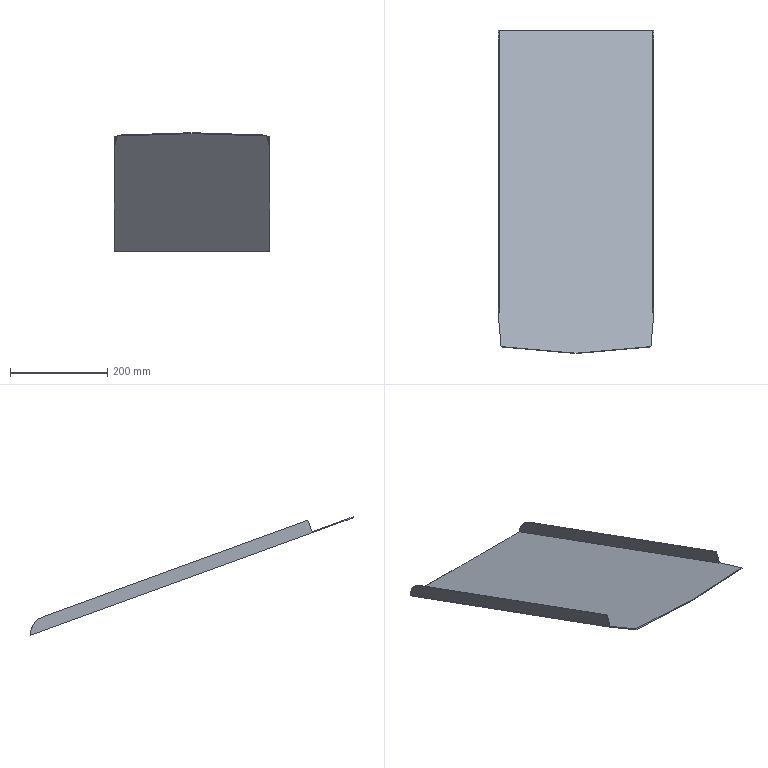Part | NX | features solid 2 | 1 solid | 16 faces | box 320 x 663.823 x 243.491 mm | volume 506723 mm3 | plane 13 | spline 2 | cylinder 1 | commonest cylinder face diameters 80 x1
STEP:
#1=CARTESIAN_POINT('',(160.,49.927,-215.652));
#2=VERTEX_POINT('',#1);
#3=CARTESIAN_POINT('',(158.,49.927,-215.652));
#4=VERTEX_POINT('',#3);
#5=CARTESIAN_POINT('',(160.,49.927,-215.652));
#6=DIRECTION('',(-1.,0.,0.));
#7=VECTOR('',#6,1000.);
#8=LINE('',#5,#7);
#9=EDGE_CURVE('',#2,#4,#8,.T.);
#10=ORIENTED_EDGE('',*,*,#9,.T.);
#11=CARTESIAN_POINT('',(158.,41.376,-239.145));
#12=VERTEX_POINT('',#11);
#13=CARTESIAN_POINT('',(158.,49.927,-215.652));
#14=DIRECTION('',(0.,-0.342,-0.9397));
#15=VECTOR('',#14,1000.);
#16=LINE('',#13,#15);
#17=EDGE_CURVE('',#4,#12,#16,.T.);
#18=ORIENTED_EDGE('',*,*,#17,.T.);
#19=CARTESIAN_POINT('',(160.,41.376,-239.145));
#20=VERTEX_POINT('',#19);
#21=CARTESIAN_POINT('',(160.,41.376,-239.145));
#22=DIRECTION('',(-1.,0.,0.));
#23=VECTOR('',#22,1000.);
#24=LINE('',#21,#23);
#25=EDGE_CURVE('',#20,#12,#24,.T.);
#26=ORIENTED_EDGE('',*,*,#25,.F.);
#27=CARTESIAN_POINT('',(160.,49.927,-215.652));
#28=DIRECTION('',(0.,-0.342,-0.9397));
#29=VECTOR('',#28,1000.);
#30=LINE('',#27,#29);
#31=EDGE_CURVE('',#2,#20,#30,.T.);
#32=ORIENTED_EDGE('',*,*,#31,.F.);
#33=EDGE_LOOP('',(#10,#18,#26,#32));
#34=FACE_BOUND('',#33,.T.);
#35=CARTESIAN_POINT('',(160.,49.927,-215.652));
#36=DIRECTION('',(0.,-0.9397,0.342));
#37=DIRECTION('',(0.,-0.342,-0.9397));
#38=AXIS2_PLACEMENT_3D('',#35,#36,#37);
#39=PLANE('',#38);
#40=ADVANCED_FACE('',(#34),#39,.T.);
#41=CARTESIAN_POINT('',(160.,40.692,-241.024));
#42=VERTEX_POINT('',#41);
#43=CARTESIAN_POINT('',(153.945,-30.355,-215.165));
#44=VERTEX_POINT('',#43);
#45=CARTESIAN_POINT('',(160.,40.692,-241.024));
#46=CARTESIAN_POINT('',(157.796,16.869,-232.353));
#47=CARTESIAN_POINT('',(155.777,-6.813,-223.734));
#48=CARTESIAN_POINT('',(153.945,-30.355,-215.165));
#49=B_SPLINE_CURVE_WITH_KNOTS('',3,(#45,#46,#47,#48),.UNSPECIFIED.,.F.,.F.,(4,4),(0.,1.),.UNSPECIFIED.);
#50=EDGE_CURVE('',#42,#44,#49,.T.);
#51=ORIENTED_EDGE('',*,*,#50,.F.);
#52=CARTESIAN_POINT('',(160.,40.692,-241.024));
#53=CARTESIAN_POINT('',(160.,40.92,-240.398));
#54=CARTESIAN_POINT('',(160.,41.148,-239.771));
#55=CARTESIAN_POINT('',(160.,41.376,-239.145));
#56=B_SPLINE_CURVE_WITH_KNOTS('',3,(#52,#53,#54,#55),.UNSPECIFIED.,.F.,.F.,(4,4),(0.,1.),.UNSPECIFIED.);
#57=EDGE_CURVE('',#20,#42,#56,.F.);
#58=ORIENTED_EDGE('',*,*,#57,.F.);
#59=CARTESIAN_POINT('',(153.945,-29.671,-213.286));
#60=VERTEX_POINT('',#59);
#61=CARTESIAN_POINT('',(160.,41.376,-239.145));
#62=CARTESIAN_POINT('',(157.796,17.553,-230.474));
#63=CARTESIAN_POINT('',(155.777,-6.129,-221.854));
#64=CARTESIAN_POINT('',(153.945,-29.671,-213.286));
#65=B_SPLINE_CURVE_WITH_KNOTS('',3,(#61,#62,#63,#64),.UNSPECIFIED.,.F.,.F.,(4,4),(0.,1.),.UNSPECIFIED.);
#66=EDGE_CURVE('',#20,#60,#65,.T.);
#67=ORIENTED_EDGE('',*,*,#66,.T.);
#68=CARTESIAN_POINT('',(153.945,-29.671,-213.286));
#69=CARTESIAN_POINT('',(153.945,-29.899,-213.912));
#70=CARTESIAN_POINT('',(153.945,-30.127,-214.539));
#71=CARTESIAN_POINT('',(153.945,-30.355,-215.165));
#72=B_SPLINE_CURVE_WITH_KNOTS('',3,(#68,#69,#70,#71),.UNSPECIFIED.,.F.,.F.,(4,4),(0.,1.),.UNSPECIFIED.);
#73=EDGE_CURVE('',#60,#44,#72,.T.);
#74=ORIENTED_EDGE('',*,*,#73,.T.);
#75=EDGE_LOOP('',(#51,#58,#67,#74));
#76=FACE_BOUND('',#75,.T.);
#77=CARTESIAN_POINT('',(160.,41.376,-239.145));
#78=CARTESIAN_POINT('',(160.,40.692,-241.024));
#79=CARTESIAN_POINT('',(157.796,17.553,-230.474));
#80=CARTESIAN_POINT('',(157.796,16.869,-232.353));
#81=CARTESIAN_POINT('',(155.777,-6.129,-221.854));
#82=CARTESIAN_POINT('',(155.777,-6.813,-223.734));
#83=CARTESIAN_POINT('',(153.945,-29.671,-213.286));
#84=CARTESIAN_POINT('',(153.945,-30.355,-215.165));
#85=B_SPLINE_SURFACE_WITH_KNOTS('',3,1,((#77,#78),(#79,#80),(#81,#82),(#83,#84)),.SURF_OF_LINEAR_EXTRUSION.,.F.,.F.,.F.,(4,4),(2,2),(0.,1.),(0.,1.),.PIECEWISE_BEZIER_KNOTS.);
#86=ADVANCED_FACE('',(#76),#85,.T.);
#87=CARTESIAN_POINT('',(158.,619.975,-449.737));
#88=VERTEX_POINT('',#87);
#89=CARTESIAN_POINT('',(158.,620.,-449.747));
#90=DIRECTION('',(0.,-0.9397,0.342));
#91=VECTOR('',#90,1000.);
#92=LINE('',#89,#91);
#93=EDGE_CURVE('',#88,#12,#92,.T.);
#94=ORIENTED_EDGE('',*,*,#93,.T.);
#95=ORIENTED_EDGE('',*,*,#17,.F.);
#96=CARTESIAN_POINT('',(158.,593.681,-413.563));
#97=VERTEX_POINT('',#96);
#98=CARTESIAN_POINT('',(158.,628.551,-426.254));
#99=DIRECTION('',(0.,-0.9397,0.342));
#100=VECTOR('',#99,1000.);
#101=LINE('',#98,#100);
#102=EDGE_CURVE('',#97,#4,#101,.T.);
#103=ORIENTED_EDGE('',*,*,#102,.F.);
#104=CARTESIAN_POINT('',(158.,580.,-451.15));
#105=DIRECTION('',(1.,0.,0.));
#106=DIRECTION('',(0.,0.,-1.));
#107=AXIS2_PLACEMENT_3D('',#104,#105,#106);
#108=CIRCLE('',#107,40.);
#109=EDGE_CURVE('',#88,#97,#108,.T.);
#110=ORIENTED_EDGE('',*,*,#109,.F.);
#111=EDGE_LOOP('',(#94,#95,#103,#110));
#112=FACE_BOUND('',#111,.T.);
#113=CARTESIAN_POINT('',(158.,628.551,-426.254));
#114=DIRECTION('',(-1.,0.,0.));
#115=DIRECTION('',(0.,0.,-1.));
#116=AXIS2_PLACEMENT_3D('',#113,#114,#115);
#117=PLANE('',#116);
#118=ADVANCED_FACE('',(#112),#117,.T.);
#119=ORIENTED_EDGE('',*,*,#102,.T.);
#120=ORIENTED_EDGE('',*,*,#9,.F.);
#121=CARTESIAN_POINT('',(160.,593.681,-413.563));
#122=VERTEX_POINT('',#121);
#123=CARTESIAN_POINT('',(160.,628.551,-426.254));
#124=DIRECTION('',(0.,-0.9397,0.342));
#125=VECTOR('',#124,1000.);
#126=LINE('',#123,#125);
#127=EDGE_CURVE('',#122,#2,#126,.T.);
#128=ORIENTED_EDGE('',*,*,#127,.F.);
#129=CARTESIAN_POINT('',(159.,593.681,-413.563));
#130=DIRECTION('',(1.,0.,0.));
#131=VECTOR('',#130,1000.);
#132=LINE('',#129,#131);
#133=EDGE_CURVE('',#97,#122,#132,.T.);
#134=ORIENTED_EDGE('',*,*,#133,.F.);
#135=EDGE_LOOP('',(#119,#120,#128,#134));
#136=FACE_BOUND('',#135,.T.);
#137=CARTESIAN_POINT('',(160.,628.551,-426.254));
#138=DIRECTION('',(0.,0.342,0.9397));
#139=DIRECTION('',(0.,-0.9397,0.342));
#140=AXIS2_PLACEMENT_3D('',#137,#138,#139);
#141=PLANE('',#140);
#142=ADVANCED_FACE('',(#136),#141,.T.);
#143=ORIENTED_EDGE('',*,*,#127,.T.);
#144=ORIENTED_EDGE('',*,*,#31,.T.);
#145=ORIENTED_EDGE('',*,*,#57,.T.);
#146=CARTESIAN_POINT('',(160.,620.,-451.875));
#147=VERTEX_POINT('',#146);
#148=CARTESIAN_POINT('',(160.,-452.731,-61.433));
#149=DIRECTION('',(0.,-0.9397,0.342));
#150=VECTOR('',#149,1000.);
#151=LINE('',#148,#150);
#152=EDGE_CURVE('',#147,#42,#151,.T.);
#153=ORIENTED_EDGE('',*,*,#152,.F.);
#154=CARTESIAN_POINT('',(160.,620.,-451.15));
#155=VERTEX_POINT('',#154);
#156=CARTESIAN_POINT('',(160.,620.,-570.));
#157=DIRECTION('',(0.,0.,1.));
#158=VECTOR('',#157,1000.);
#159=LINE('',#156,#158);
#160=EDGE_CURVE('',#155,#147,#159,.F.);
#161=ORIENTED_EDGE('',*,*,#160,.F.);
#162=CARTESIAN_POINT('',(160.,580.,-451.15));
#163=DIRECTION('',(1.,0.,0.));
#164=DIRECTION('',(0.,0.,-1.));
#165=AXIS2_PLACEMENT_3D('',#162,#163,#164);
#166=CIRCLE('',#165,40.);
#167=EDGE_CURVE('',#122,#155,#166,.F.);
#168=ORIENTED_EDGE('',*,*,#167,.F.);
#169=EDGE_LOOP('',(#143,#144,#145,#153,#161,#168));
#170=FACE_BOUND('',#169,.T.);
#171=CARTESIAN_POINT('',(160.,-452.047,-59.553));
#172=DIRECTION('',(-1.,0.,0.));
#173=DIRECTION('',(0.,0.,-1.));
#174=AXIS2_PLACEMENT_3D('',#171,#172,#173);
#175=PLANE('',#174);
#176=ADVANCED_FACE('',(#170),#175,.F.);
#177=CARTESIAN_POINT('',(0.,-43.823,-210.263));
#178=VERTEX_POINT('',#177);
#179=CARTESIAN_POINT('',(619.523,10.378,-229.991));
#180=DIRECTION('',(0.9957,0.08711,-0.03171));
#181=VECTOR('',#180,1000.);
#182=LINE('',#179,#181);
#183=EDGE_CURVE('',#178,#44,#182,.T.);
#184=ORIENTED_EDGE('',*,*,#183,.F.);
#185=CARTESIAN_POINT('',(-153.945,-30.355,-215.165));
#186=VERTEX_POINT('',#185);
#187=CARTESIAN_POINT('',(-619.523,10.378,-229.991));
#188=DIRECTION('',(-0.9957,0.08711,-0.03171));
#189=VECTOR('',#188,1000.);
#190=LINE('',#187,#189);
#191=EDGE_CURVE('',#178,#186,#190,.T.);
#192=ORIENTED_EDGE('',*,*,#191,.T.);
#193=CARTESIAN_POINT('',(-160.,40.692,-241.024));
#194=VERTEX_POINT('',#193);
#195=CARTESIAN_POINT('',(-160.,40.692,-241.024));
#196=CARTESIAN_POINT('',(-157.796,16.869,-232.353));
#197=CARTESIAN_POINT('',(-155.777,-6.813,-223.734));
#198=CARTESIAN_POINT('',(-153.945,-30.355,-215.165));
#199=B_SPLINE_CURVE_WITH_KNOTS('',3,(#195,#196,#197,#198),.UNSPECIFIED.,.F.,.F.,(4,4),(0.,1.),.UNSPECIFIED.);
#200=EDGE_CURVE('',#194,#186,#199,.T.);
#201=ORIENTED_EDGE('',*,*,#200,.F.);
#202=CARTESIAN_POINT('',(-160.,620.,-451.875));
#203=VERTEX_POINT('',#202);
#204=CARTESIAN_POINT('',(-160.,-452.731,-61.433));
#205=DIRECTION('',(0.,-0.9397,0.342));
#206=VECTOR('',#205,1000.);
#207=LINE('',#204,#206);
#208=EDGE_CURVE('',#203,#194,#207,.T.);
#209=ORIENTED_EDGE('',*,*,#208,.F.);
#210=CARTESIAN_POINT('',(-50.,620.,-451.875));
#211=DIRECTION('',(1.,0.,0.));
#212=VECTOR('',#211,1000.);
#213=LINE('',#210,#212);
#214=EDGE_CURVE('',#147,#203,#213,.F.);
#215=ORIENTED_EDGE('',*,*,#214,.F.);
#216=ORIENTED_EDGE('',*,*,#152,.T.);
#217=ORIENTED_EDGE('',*,*,#50,.T.);
#218=EDGE_LOOP('',(#184,#192,#201,#209,#215,#216,#217));
#219=FACE_BOUND('',#218,.T.);
#220=CARTESIAN_POINT('',(665.408,-452.731,-61.433));
#221=DIRECTION('',(0.,0.342,0.9397));
#222=DIRECTION('',(-1.,0.,0.));
#223=AXIS2_PLACEMENT_3D('',#220,#221,#222);
#224=PLANE('',#223);
#225=ADVANCED_FACE('',(#219),#224,.F.);
#226=CARTESIAN_POINT('',(-158.,619.975,-449.737));
#227=VERTEX_POINT('',#226);
#228=CARTESIAN_POINT('',(-258.,619.975,-449.737));
#229=DIRECTION('',(1.,0.,0.));
#230=VECTOR('',#229,1000.);
#231=LINE('',#228,#230);
#232=EDGE_CURVE('',#227,#88,#231,.T.);
#233=ORIENTED_EDGE('',*,*,#232,.T.);
#234=ORIENTED_EDGE('',*,*,#109,.T.);
#235=ORIENTED_EDGE('',*,*,#133,.T.);
#236=ORIENTED_EDGE('',*,*,#167,.T.);
#237=CARTESIAN_POINT('',(-160.,620.,-451.15));
#238=VERTEX_POINT('',#237);
#239=CARTESIAN_POINT('',(-260.,620.,-451.15));
#240=DIRECTION('',(1.,0.,0.));
#241=VECTOR('',#240,1000.);
#242=LINE('',#239,#241);
#243=EDGE_CURVE('',#155,#238,#242,.F.);
#244=ORIENTED_EDGE('',*,*,#243,.T.);
#245=CARTESIAN_POINT('',(-160.,593.681,-413.563));
#246=VERTEX_POINT('',#245);
#247=CARTESIAN_POINT('',(-160.,580.,-451.15));
#248=DIRECTION('',(1.,0.,0.));
#249=DIRECTION('',(0.,0.,-1.));
#250=AXIS2_PLACEMENT_3D('',#247,#248,#249);
#251=CIRCLE('',#250,40.);
#252=EDGE_CURVE('',#246,#238,#251,.F.);
#253=ORIENTED_EDGE('',*,*,#252,.F.);
#254=CARTESIAN_POINT('',(-158.,593.681,-413.563));
#255=VERTEX_POINT('',#254);
#256=CARTESIAN_POINT('',(-159.,593.681,-413.563));
#257=DIRECTION('',(-1.,0.,0.));
#258=VECTOR('',#257,1000.);
#259=LINE('',#256,#258);
#260=EDGE_CURVE('',#255,#246,#259,.T.);
#261=ORIENTED_EDGE('',*,*,#260,.F.);
#262=CARTESIAN_POINT('',(-158.,580.,-451.15));
#263=DIRECTION('',(1.,0.,0.));
#264=DIRECTION('',(0.,0.,-1.));
#265=AXIS2_PLACEMENT_3D('',#262,#263,#264);
#266=CIRCLE('',#265,40.);
#267=EDGE_CURVE('',#227,#255,#266,.T.);
#268=ORIENTED_EDGE('',*,*,#267,.F.);
#269=EDGE_LOOP('',(#233,#234,#235,#236,#244,#253,#261,#268));
#270=FACE_BOUND('',#269,.T.);
#271=CARTESIAN_POINT('',(-260.,580.,-451.15));
#272=DIRECTION('',(1.,0.,0.));
#273=DIRECTION('',(0.,0.,1.));
#274=AXIS2_PLACEMENT_3D('',#271,#272,#273);
#275=CYLINDRICAL_SURFACE('',#274,40.);
#276=ADVANCED_FACE('',(#270),#275,.T.);
#277=ORIENTED_EDGE('',*,*,#243,.F.);
#278=ORIENTED_EDGE('',*,*,#160,.T.);
#279=ORIENTED_EDGE('',*,*,#214,.T.);
#280=CARTESIAN_POINT('',(-160.,620.,-570.));
#281=DIRECTION('',(0.,0.,1.));
#282=VECTOR('',#281,1000.);
#283=LINE('',#280,#282);
#284=EDGE_CURVE('',#238,#203,#283,.F.);
#285=ORIENTED_EDGE('',*,*,#284,.F.);
#286=EDGE_LOOP('',(#277,#278,#279,#285));
#287=FACE_BOUND('',#286,.T.);
#288=CARTESIAN_POINT('',(-50.,620.,-570.));
#289=DIRECTION('',(0.,-1.,0.));
#290=DIRECTION('',(1.,0.,0.));
#291=AXIS2_PLACEMENT_3D('',#288,#289,#290);
#292=PLANE('',#291);
#293=ADVANCED_FACE('',(#287),#292,.F.);
#294=ORIENTED_EDGE('',*,*,#183,.T.);
#295=ORIENTED_EDGE('',*,*,#73,.F.);
#296=CARTESIAN_POINT('',(0.,-43.139,-208.384));
#297=VERTEX_POINT('',#296);
#298=CARTESIAN_POINT('',(619.523,11.062,-228.111));
#299=DIRECTION('',(0.9957,0.08711,-0.03171));
#300=VECTOR('',#299,1000.);
#301=LINE('',#298,#300);
#302=EDGE_CURVE('',#297,#60,#301,.T.);
#303=ORIENTED_EDGE('',*,*,#302,.F.);
#304=CARTESIAN_POINT('',(0.,28.88,-10.512));
#305=DIRECTION('',(0.,-0.342,-0.9397));
#306=VECTOR('',#305,1000.);
#307=LINE('',#304,#306);
#308=EDGE_CURVE('',#297,#178,#307,.T.);
#309=ORIENTED_EDGE('',*,*,#308,.T.);
#310=EDGE_LOOP('',(#294,#295,#303,#309));
#311=FACE_BOUND('',#310,.T.);
#312=CARTESIAN_POINT('',(619.523,11.062,-228.111));
#313=DIRECTION('',(0.0927,-0.9356,0.3405));
#314=DIRECTION('',(0.,-0.342,-0.9397));
#315=AXIS2_PLACEMENT_3D('',#312,#313,#314);
#316=PLANE('',#315);
#317=ADVANCED_FACE('',(#311),#316,.T.);
#318=ORIENTED_EDGE('',*,*,#302,.T.);
#319=ORIENTED_EDGE('',*,*,#66,.F.);
#320=ORIENTED_EDGE('',*,*,#25,.T.);
#321=ORIENTED_EDGE('',*,*,#93,.F.);
#322=ORIENTED_EDGE('',*,*,#232,.F.);
#323=CARTESIAN_POINT('',(-158.,41.376,-239.145));
#324=VERTEX_POINT('',#323);
#325=CARTESIAN_POINT('',(-158.,620.,-449.747));
#326=DIRECTION('',(0.,-0.9397,0.342));
#327=VECTOR('',#326,1000.);
#328=LINE('',#325,#327);
#329=EDGE_CURVE('',#227,#324,#328,.T.);
#330=ORIENTED_EDGE('',*,*,#329,.T.);
#331=CARTESIAN_POINT('',(-160.,41.376,-239.145));
#332=VERTEX_POINT('',#331);
#333=CARTESIAN_POINT('',(-160.,41.376,-239.145));
#334=DIRECTION('',(1.,0.,0.));
#335=VECTOR('',#334,1000.);
#336=LINE('',#333,#335);
#337=EDGE_CURVE('',#332,#324,#336,.T.);
#338=ORIENTED_EDGE('',*,*,#337,.F.);
#339=CARTESIAN_POINT('',(-153.945,-29.671,-213.286));
#340=VERTEX_POINT('',#339);
#341=CARTESIAN_POINT('',(-160.,41.376,-239.145));
#342=CARTESIAN_POINT('',(-157.796,17.553,-230.474));
#343=CARTESIAN_POINT('',(-155.777,-6.129,-221.854));
#344=CARTESIAN_POINT('',(-153.945,-29.671,-213.286));
#345=B_SPLINE_CURVE_WITH_KNOTS('',3,(#341,#342,#343,#344),.UNSPECIFIED.,.F.,.F.,(4,4),(0.,1.),.UNSPECIFIED.);
#346=EDGE_CURVE('',#332,#340,#345,.T.);
#347=ORIENTED_EDGE('',*,*,#346,.T.);
#348=CARTESIAN_POINT('',(-619.523,11.062,-228.111));
#349=DIRECTION('',(-0.9957,0.08711,-0.03171));
#350=VECTOR('',#349,1000.);
#351=LINE('',#348,#350);
#352=EDGE_CURVE('',#297,#340,#351,.T.);
#353=ORIENTED_EDGE('',*,*,#352,.F.);
#354=EDGE_LOOP('',(#318,#319,#320,#321,#322,#330,#338,#347,#353));
#355=FACE_BOUND('',#354,.T.);
#356=CARTESIAN_POINT('',(665.408,-452.047,-59.553));
#357=DIRECTION('',(0.,0.342,0.9397));
#358=DIRECTION('',(-1.,0.,0.));
#359=AXIS2_PLACEMENT_3D('',#356,#357,#358);
#360=PLANE('',#359);
#361=ADVANCED_FACE('',(#355),#360,.T.);
#362=CARTESIAN_POINT('',(-160.,49.927,-215.652));
#363=VERTEX_POINT('',#362);
#364=CARTESIAN_POINT('',(-158.,49.927,-215.652));
#365=VERTEX_POINT('',#364);
#366=CARTESIAN_POINT('',(-160.,49.927,-215.652));
#367=DIRECTION('',(1.,0.,0.));
#368=VECTOR('',#367,1000.);
#369=LINE('',#366,#368);
#370=EDGE_CURVE('',#363,#365,#369,.T.);
#371=ORIENTED_EDGE('',*,*,#370,.F.);
#372=CARTESIAN_POINT('',(-160.,49.927,-215.652));
#373=DIRECTION('',(0.,-0.342,-0.9397));
#374=VECTOR('',#373,1000.);
#375=LINE('',#372,#374);
#376=EDGE_CURVE('',#363,#332,#375,.T.);
#377=ORIENTED_EDGE('',*,*,#376,.T.);
#378=ORIENTED_EDGE('',*,*,#337,.T.);
#379=CARTESIAN_POINT('',(-158.,49.927,-215.652));
#380=DIRECTION('',(0.,-0.342,-0.9397));
#381=VECTOR('',#380,1000.);
#382=LINE('',#379,#381);
#383=EDGE_CURVE('',#365,#324,#382,.T.);
#384=ORIENTED_EDGE('',*,*,#383,.F.);
#385=EDGE_LOOP('',(#371,#377,#378,#384));
#386=FACE_BOUND('',#385,.T.);
#387=CARTESIAN_POINT('',(-160.,49.927,-215.652));
#388=DIRECTION('',(0.,-0.9397,0.342));
#389=DIRECTION('',(0.,-0.342,-0.9397));
#390=AXIS2_PLACEMENT_3D('',#387,#388,#389);
#391=PLANE('',#390);
#392=ADVANCED_FACE('',(#386),#391,.T.);
#393=ORIENTED_EDGE('',*,*,#200,.T.);
#394=CARTESIAN_POINT('',(-153.945,-29.671,-213.286));
#395=CARTESIAN_POINT('',(-153.945,-29.899,-213.912));
#396=CARTESIAN_POINT('',(-153.945,-30.127,-214.539));
#397=CARTESIAN_POINT('',(-153.945,-30.355,-215.165));
#398=B_SPLINE_CURVE_WITH_KNOTS('',3,(#394,#395,#396,#397),.UNSPECIFIED.,.F.,.F.,(4,4),(0.,1.),.UNSPECIFIED.);
#399=EDGE_CURVE('',#340,#186,#398,.T.);
#400=ORIENTED_EDGE('',*,*,#399,.F.);
#401=ORIENTED_EDGE('',*,*,#346,.F.);
#402=CARTESIAN_POINT('',(-160.,40.692,-241.024));
#403=CARTESIAN_POINT('',(-160.,40.92,-240.398));
#404=CARTESIAN_POINT('',(-160.,41.148,-239.771));
#405=CARTESIAN_POINT('',(-160.,41.376,-239.145));
#406=B_SPLINE_CURVE_WITH_KNOTS('',3,(#402,#403,#404,#405),.UNSPECIFIED.,.F.,.F.,(4,4),(0.,1.),.UNSPECIFIED.);
#407=EDGE_CURVE('',#332,#194,#406,.F.);
#408=ORIENTED_EDGE('',*,*,#407,.T.);
#409=EDGE_LOOP('',(#393,#400,#401,#408));
#410=FACE_BOUND('',#409,.T.);
#411=CARTESIAN_POINT('',(-160.,41.376,-239.145));
#412=CARTESIAN_POINT('',(-160.,40.692,-241.024));
#413=CARTESIAN_POINT('',(-157.796,17.553,-230.474));
#414=CARTESIAN_POINT('',(-157.796,16.869,-232.353));
#415=CARTESIAN_POINT('',(-155.777,-6.129,-221.854));
#416=CARTESIAN_POINT('',(-155.777,-6.813,-223.734));
#417=CARTESIAN_POINT('',(-153.945,-29.671,-213.286));
#418=CARTESIAN_POINT('',(-153.945,-30.355,-215.165));
#419=B_SPLINE_SURFACE_WITH_KNOTS('',3,1,((#411,#412),(#413,#414),(#415,#416),(#417,#418)),.SURF_OF_LINEAR_EXTRUSION.,.F.,.F.,.F.,(4,4),(2,2),(0.,1.),(0.,1.),.PIECEWISE_BEZIER_KNOTS.);
#420=ADVANCED_FACE('',(#410),#419,.F.);
#421=ORIENTED_EDGE('',*,*,#329,.F.);
#422=ORIENTED_EDGE('',*,*,#267,.T.);
#423=CARTESIAN_POINT('',(-158.,628.551,-426.254));
#424=DIRECTION('',(0.,-0.9397,0.342));
#425=VECTOR('',#424,1000.);
#426=LINE('',#423,#425);
#427=EDGE_CURVE('',#255,#365,#426,.T.);
#428=ORIENTED_EDGE('',*,*,#427,.T.);
#429=ORIENTED_EDGE('',*,*,#383,.T.);
#430=EDGE_LOOP('',(#421,#422,#428,#429));
#431=FACE_BOUND('',#430,.T.);
#432=CARTESIAN_POINT('',(-158.,628.551,-426.254));
#433=DIRECTION('',(1.,0.,0.));
#434=DIRECTION('',(0.,0.,-1.));
#435=AXIS2_PLACEMENT_3D('',#432,#433,#434);
#436=PLANE('',#435);
#437=ADVANCED_FACE('',(#431),#436,.T.);
#438=ORIENTED_EDGE('',*,*,#427,.F.);
#439=ORIENTED_EDGE('',*,*,#260,.T.);
#440=CARTESIAN_POINT('',(-160.,628.551,-426.254));
#441=DIRECTION('',(0.,-0.9397,0.342));
#442=VECTOR('',#441,1000.);
#443=LINE('',#440,#442);
#444=EDGE_CURVE('',#246,#363,#443,.T.);
#445=ORIENTED_EDGE('',*,*,#444,.T.);
#446=ORIENTED_EDGE('',*,*,#370,.T.);
#447=EDGE_LOOP('',(#438,#439,#445,#446));
#448=FACE_BOUND('',#447,.T.);
#449=CARTESIAN_POINT('',(-160.,628.551,-426.254));
#450=DIRECTION('',(0.,0.342,0.9397));
#451=DIRECTION('',(0.,-0.9397,0.342));
#452=AXIS2_PLACEMENT_3D('',#449,#450,#451);
#453=PLANE('',#452);
#454=ADVANCED_FACE('',(#448),#453,.T.);
#455=ORIENTED_EDGE('',*,*,#444,.F.);
#456=ORIENTED_EDGE('',*,*,#252,.T.);
#457=ORIENTED_EDGE('',*,*,#284,.T.);
#458=ORIENTED_EDGE('',*,*,#208,.T.);
#459=ORIENTED_EDGE('',*,*,#407,.F.);
#460=ORIENTED_EDGE('',*,*,#376,.F.);
#461=EDGE_LOOP('',(#455,#456,#457,#458,#459,#460));
#462=FACE_BOUND('',#461,.T.);
#463=CARTESIAN_POINT('',(-160.,-452.047,-59.553));
#464=DIRECTION('',(1.,0.,0.));
#465=DIRECTION('',(0.,0.,-1.));
#466=AXIS2_PLACEMENT_3D('',#463,#464,#465);
#467=PLANE('',#466);
#468=ADVANCED_FACE('',(#462),#467,.F.);
#469=ORIENTED_EDGE('',*,*,#191,.F.);
#470=ORIENTED_EDGE('',*,*,#308,.F.);
#471=ORIENTED_EDGE('',*,*,#352,.T.);
#472=ORIENTED_EDGE('',*,*,#399,.T.);
#473=EDGE_LOOP('',(#469,#470,#471,#472));
#474=FACE_BOUND('',#473,.T.);
#475=CARTESIAN_POINT('',(-619.523,11.062,-228.111));
#476=DIRECTION('',(-0.0927,-0.9356,0.3405));
#477=DIRECTION('',(0.,-0.342,-0.9397));
#478=AXIS2_PLACEMENT_3D('',#475,#476,#477);
#479=PLANE('',#478);
#480=ADVANCED_FACE('',(#474),#479,.T.);
#481=CLOSED_SHELL('',(#40,#86,#118,#142,#176,#225,#276,#293,#317,#361,#392,#420,#437,#454,#468,#480));
#482=MANIFOLD_SOLID_BREP('',#481);
#483=(LENGTH_UNIT()NAMED_UNIT(*)SI_UNIT(.MILLI.,.METRE.));
#484=UNCERTAINTY_MEASURE_WITH_UNIT(LENGTH_MEASURE(0.0508),#483,'','');
#485=(NAMED_UNIT(*)PLANE_ANGLE_UNIT()SI_UNIT($,.RADIAN.));
#486=(NAMED_UNIT(*)SI_UNIT($,.STERADIAN.)SOLID_ANGLE_UNIT());
#487=(GEOMETRIC_REPRESENTATION_CONTEXT(3)GLOBAL_UNCERTAINTY_ASSIGNED_CONTEXT((#484))GLOBAL_UNIT_ASSIGNED_CONTEXT((#483,#485,#486))REPRESENTATION_CONTEXT('',''));
#488=ADVANCED_BREP_SHAPE_REPRESENTATION('',(#482),#487);